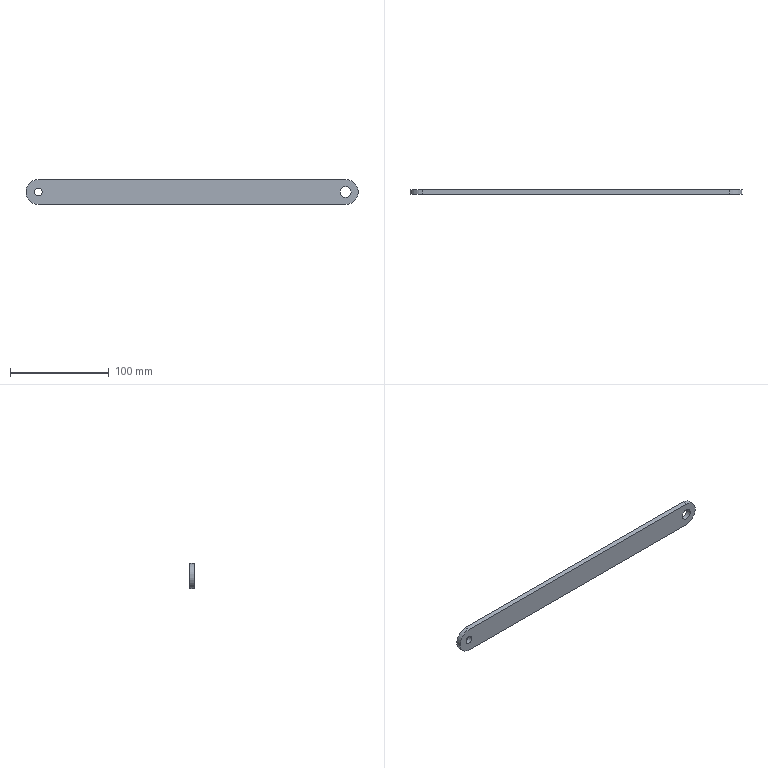Part | NX | features BREP 1 | 1 solid | 10 faces | box 336.55 x 4.763 x 25.4 mm | volume 39340 mm3 | cylinder 6 | plane 4 | commonest cylinder face diameters 8.128 x2 11.151 x2 25.4 x2
STEP:
#1=CARTESIAN_POINT('',(-155.575,0.,12.7));
#2=VERTEX_POINT('',#1);
#3=CARTESIAN_POINT('',(155.575,0.,12.7));
#4=VERTEX_POINT('',#3);
#5=CARTESIAN_POINT('',(-155.575,0.,12.7));
#6=DIRECTION('',(1.,0.,0.));
#7=VECTOR('',#6,1000.);
#8=LINE('',#5,#7);
#9=EDGE_CURVE('',#2,#4,#8,.T.);
#10=ORIENTED_EDGE('',*,*,#9,.T.);
#11=CARTESIAN_POINT('',(155.575,0.,-12.7));
#12=VERTEX_POINT('',#11);
#13=CARTESIAN_POINT('',(155.575,0.,0.));
#14=DIRECTION('',(0.,1.,0.));
#15=DIRECTION('',(0.,0.,1.));
#16=AXIS2_PLACEMENT_3D('',#13,#14,#15);
#17=CIRCLE('',#16,12.7);
#18=EDGE_CURVE('',#4,#12,#17,.T.);
#19=ORIENTED_EDGE('',*,*,#18,.T.);
#20=CARTESIAN_POINT('',(-155.575,0.,-12.7));
#21=VERTEX_POINT('',#20);
#22=CARTESIAN_POINT('',(155.575,0.,-12.7));
#23=DIRECTION('',(-1.,0.,0.));
#24=VECTOR('',#23,1000.);
#25=LINE('',#22,#24);
#26=EDGE_CURVE('',#12,#21,#25,.T.);
#27=ORIENTED_EDGE('',*,*,#26,.T.);
#28=CARTESIAN_POINT('',(-155.575,0.,0.));
#29=DIRECTION('',(0.,1.,0.));
#30=DIRECTION('',(0.,0.,-1.));
#31=AXIS2_PLACEMENT_3D('',#28,#29,#30);
#32=CIRCLE('',#31,12.7);
#33=EDGE_CURVE('',#21,#2,#32,.T.);
#34=ORIENTED_EDGE('',*,*,#33,.T.);
#35=EDGE_LOOP('',(#10,#19,#27,#34));
#36=FACE_BOUND('',#35,.T.);
#37=CARTESIAN_POINT('',(150.,0.,0.));
#38=VERTEX_POINT('',#37);
#39=CARTESIAN_POINT('',(161.15,0.,0.));
#40=VERTEX_POINT('',#39);
#41=CARTESIAN_POINT('',(155.575,0.,0.));
#42=DIRECTION('',(0.,-1.,0.));
#43=DIRECTION('',(-1.,0.,0.));
#44=AXIS2_PLACEMENT_3D('',#41,#42,#43);
#45=CIRCLE('',#44,5.575);
#46=EDGE_CURVE('',#38,#40,#45,.T.);
#47=ORIENTED_EDGE('',*,*,#46,.T.);
#48=CARTESIAN_POINT('',(155.575,0.,0.));
#49=DIRECTION('',(0.,-1.,0.));
#50=DIRECTION('',(1.,0.,0.));
#51=AXIS2_PLACEMENT_3D('',#48,#49,#50);
#52=CIRCLE('',#51,5.575);
#53=EDGE_CURVE('',#40,#38,#52,.T.);
#54=ORIENTED_EDGE('',*,*,#53,.T.);
#55=EDGE_LOOP('',(#47,#54));
#56=FACE_BOUND('',#55,.T.);
#57=CARTESIAN_POINT('',(-159.639,0.,0.));
#58=VERTEX_POINT('',#57);
#59=CARTESIAN_POINT('',(-151.511,0.,0.));
#60=VERTEX_POINT('',#59);
#61=CARTESIAN_POINT('',(-155.575,0.,0.));
#62=DIRECTION('',(0.,-1.,0.));
#63=DIRECTION('',(-1.,0.,0.));
#64=AXIS2_PLACEMENT_3D('',#61,#62,#63);
#65=CIRCLE('',#64,4.064);
#66=EDGE_CURVE('',#58,#60,#65,.T.);
#67=ORIENTED_EDGE('',*,*,#66,.T.);
#68=CARTESIAN_POINT('',(-155.575,0.,0.));
#69=DIRECTION('',(0.,-1.,0.));
#70=DIRECTION('',(1.,0.,0.));
#71=AXIS2_PLACEMENT_3D('',#68,#69,#70);
#72=CIRCLE('',#71,4.064);
#73=EDGE_CURVE('',#60,#58,#72,.T.);
#74=ORIENTED_EDGE('',*,*,#73,.T.);
#75=EDGE_LOOP('',(#67,#74));
#76=FACE_BOUND('',#75,.T.);
#77=CARTESIAN_POINT('',(0.,0.,0.));
#78=DIRECTION('',(0.,1.,0.));
#79=DIRECTION('',(1.,0.,0.));
#80=AXIS2_PLACEMENT_3D('',#77,#78,#79);
#81=PLANE('',#80);
#82=ADVANCED_FACE('',(#36,#56,#76),#81,.T.);
#83=CARTESIAN_POINT('',(-155.575,-4.763,-12.7));
#84=VERTEX_POINT('',#83);
#85=CARTESIAN_POINT('',(-155.575,0.,-12.7));
#86=DIRECTION('',(0.,-1.,0.));
#87=VECTOR('',#86,1000.);
#88=LINE('',#85,#87);
#89=EDGE_CURVE('',#21,#84,#88,.T.);
#90=ORIENTED_EDGE('',*,*,#89,.T.);
#91=CARTESIAN_POINT('',(-155.575,-4.763,12.7));
#92=VERTEX_POINT('',#91);
#93=CARTESIAN_POINT('',(-155.575,-4.763,0.));
#94=DIRECTION('',(0.,1.,0.));
#95=DIRECTION('',(0.,0.,-1.));
#96=AXIS2_PLACEMENT_3D('',#93,#94,#95);
#97=CIRCLE('',#96,12.7);
#98=EDGE_CURVE('',#84,#92,#97,.T.);
#99=ORIENTED_EDGE('',*,*,#98,.T.);
#100=CARTESIAN_POINT('',(-155.575,0.,12.7));
#101=DIRECTION('',(0.,-1.,0.));
#102=VECTOR('',#101,1000.);
#103=LINE('',#100,#102);
#104=EDGE_CURVE('',#2,#92,#103,.T.);
#105=ORIENTED_EDGE('',*,*,#104,.F.);
#106=ORIENTED_EDGE('',*,*,#33,.F.);
#107=EDGE_LOOP('',(#90,#99,#105,#106));
#108=FACE_BOUND('',#107,.T.);
#109=CARTESIAN_POINT('',(-155.575,-2.381,0.));
#110=DIRECTION('',(0.,1.,0.));
#111=DIRECTION('',(0.,0.,-1.));
#112=AXIS2_PLACEMENT_3D('',#109,#110,#111);
#113=CYLINDRICAL_SURFACE('',#112,12.7);
#114=ADVANCED_FACE('',(#108),#113,.T.);
#115=ORIENTED_EDGE('',*,*,#104,.T.);
#116=CARTESIAN_POINT('',(155.575,-4.763,12.7));
#117=VERTEX_POINT('',#116);
#118=CARTESIAN_POINT('',(-155.575,-4.763,12.7));
#119=DIRECTION('',(1.,0.,0.));
#120=VECTOR('',#119,1000.);
#121=LINE('',#118,#120);
#122=EDGE_CURVE('',#92,#117,#121,.T.);
#123=ORIENTED_EDGE('',*,*,#122,.T.);
#124=CARTESIAN_POINT('',(155.575,0.,12.7));
#125=DIRECTION('',(0.,-1.,0.));
#126=VECTOR('',#125,1000.);
#127=LINE('',#124,#126);
#128=EDGE_CURVE('',#4,#117,#127,.T.);
#129=ORIENTED_EDGE('',*,*,#128,.F.);
#130=ORIENTED_EDGE('',*,*,#9,.F.);
#131=EDGE_LOOP('',(#115,#123,#129,#130));
#132=FACE_BOUND('',#131,.T.);
#133=CARTESIAN_POINT('',(0.,-2.381,12.7));
#134=DIRECTION('',(0.,0.,1.));
#135=DIRECTION('',(1.,0.,0.));
#136=AXIS2_PLACEMENT_3D('',#133,#134,#135);
#137=PLANE('',#136);
#138=ADVANCED_FACE('',(#132),#137,.T.);
#139=ORIENTED_EDGE('',*,*,#128,.T.);
#140=CARTESIAN_POINT('',(155.575,-4.763,-12.7));
#141=VERTEX_POINT('',#140);
#142=CARTESIAN_POINT('',(155.575,-4.763,0.));
#143=DIRECTION('',(0.,1.,0.));
#144=DIRECTION('',(0.,0.,1.));
#145=AXIS2_PLACEMENT_3D('',#142,#143,#144);
#146=CIRCLE('',#145,12.7);
#147=EDGE_CURVE('',#117,#141,#146,.T.);
#148=ORIENTED_EDGE('',*,*,#147,.T.);
#149=CARTESIAN_POINT('',(155.575,0.,-12.7));
#150=DIRECTION('',(0.,-1.,0.));
#151=VECTOR('',#150,1000.);
#152=LINE('',#149,#151);
#153=EDGE_CURVE('',#12,#141,#152,.T.);
#154=ORIENTED_EDGE('',*,*,#153,.F.);
#155=ORIENTED_EDGE('',*,*,#18,.F.);
#156=EDGE_LOOP('',(#139,#148,#154,#155));
#157=FACE_BOUND('',#156,.T.);
#158=CARTESIAN_POINT('',(155.575,-2.381,0.));
#159=DIRECTION('',(0.,1.,0.));
#160=DIRECTION('',(0.,0.,1.));
#161=AXIS2_PLACEMENT_3D('',#158,#159,#160);
#162=CYLINDRICAL_SURFACE('',#161,12.7);
#163=ADVANCED_FACE('',(#157),#162,.T.);
#164=ORIENTED_EDGE('',*,*,#153,.T.);
#165=CARTESIAN_POINT('',(155.575,-4.763,-12.7));
#166=DIRECTION('',(-1.,0.,0.));
#167=VECTOR('',#166,1000.);
#168=LINE('',#165,#167);
#169=EDGE_CURVE('',#141,#84,#168,.T.);
#170=ORIENTED_EDGE('',*,*,#169,.T.);
#171=ORIENTED_EDGE('',*,*,#89,.F.);
#172=ORIENTED_EDGE('',*,*,#26,.F.);
#173=EDGE_LOOP('',(#164,#170,#171,#172));
#174=FACE_BOUND('',#173,.T.);
#175=CARTESIAN_POINT('',(0.,-2.381,-12.7));
#176=DIRECTION('',(0.,0.,-1.));
#177=DIRECTION('',(0.,-1.,0.));
#178=AXIS2_PLACEMENT_3D('',#175,#176,#177);
#179=PLANE('',#178);
#180=ADVANCED_FACE('',(#174),#179,.T.);
#181=ORIENTED_EDGE('',*,*,#169,.F.);
#182=ORIENTED_EDGE('',*,*,#147,.F.);
#183=ORIENTED_EDGE('',*,*,#122,.F.);
#184=ORIENTED_EDGE('',*,*,#98,.F.);
#185=EDGE_LOOP('',(#181,#182,#183,#184));
#186=FACE_BOUND('',#185,.T.);
#187=CARTESIAN_POINT('',(150.,-4.763,0.));
#188=VERTEX_POINT('',#187);
#189=CARTESIAN_POINT('',(161.15,-4.763,0.));
#190=VERTEX_POINT('',#189);
#191=CARTESIAN_POINT('',(155.575,-4.763,0.));
#192=DIRECTION('',(0.,-1.,0.));
#193=DIRECTION('',(-1.,0.,0.));
#194=AXIS2_PLACEMENT_3D('',#191,#192,#193);
#195=CIRCLE('',#194,5.575);
#196=EDGE_CURVE('',#188,#190,#195,.T.);
#197=ORIENTED_EDGE('',*,*,#196,.F.);
#198=CARTESIAN_POINT('',(155.575,-4.763,0.));
#199=DIRECTION('',(0.,-1.,0.));
#200=DIRECTION('',(1.,0.,0.));
#201=AXIS2_PLACEMENT_3D('',#198,#199,#200);
#202=CIRCLE('',#201,5.575);
#203=EDGE_CURVE('',#190,#188,#202,.T.);
#204=ORIENTED_EDGE('',*,*,#203,.F.);
#205=EDGE_LOOP('',(#197,#204));
#206=FACE_BOUND('',#205,.T.);
#207=CARTESIAN_POINT('',(-159.639,-4.763,0.));
#208=VERTEX_POINT('',#207);
#209=CARTESIAN_POINT('',(-151.511,-4.763,0.));
#210=VERTEX_POINT('',#209);
#211=CARTESIAN_POINT('',(-155.575,-4.763,0.));
#212=DIRECTION('',(0.,-1.,0.));
#213=DIRECTION('',(-1.,0.,0.));
#214=AXIS2_PLACEMENT_3D('',#211,#212,#213);
#215=CIRCLE('',#214,4.064);
#216=EDGE_CURVE('',#208,#210,#215,.T.);
#217=ORIENTED_EDGE('',*,*,#216,.F.);
#218=CARTESIAN_POINT('',(-155.575,-4.763,0.));
#219=DIRECTION('',(0.,-1.,0.));
#220=DIRECTION('',(1.,0.,0.));
#221=AXIS2_PLACEMENT_3D('',#218,#219,#220);
#222=CIRCLE('',#221,4.064);
#223=EDGE_CURVE('',#210,#208,#222,.T.);
#224=ORIENTED_EDGE('',*,*,#223,.F.);
#225=EDGE_LOOP('',(#217,#224));
#226=FACE_BOUND('',#225,.T.);
#227=CARTESIAN_POINT('',(0.,-4.763,0.));
#228=DIRECTION('',(0.,1.,0.));
#229=DIRECTION('',(1.,0.,0.));
#230=AXIS2_PLACEMENT_3D('',#227,#228,#229);
#231=PLANE('',#230);
#232=ADVANCED_FACE('',(#186,#206,#226),#231,.F.);
#233=CARTESIAN_POINT('',(161.15,0.,0.));
#234=DIRECTION('',(0.,-1.,0.));
#235=VECTOR('',#234,1000.);
#236=LINE('',#233,#235);
#237=EDGE_CURVE('',#190,#40,#236,.F.);
#238=ORIENTED_EDGE('',*,*,#237,.F.);
#239=ORIENTED_EDGE('',*,*,#203,.T.);
#240=CARTESIAN_POINT('',(150.,0.,0.));
#241=DIRECTION('',(0.,-1.,0.));
#242=VECTOR('',#241,1000.);
#243=LINE('',#240,#242);
#244=EDGE_CURVE('',#188,#38,#243,.F.);
#245=ORIENTED_EDGE('',*,*,#244,.T.);
#246=ORIENTED_EDGE('',*,*,#53,.F.);
#247=EDGE_LOOP('',(#238,#239,#245,#246));
#248=FACE_BOUND('',#247,.T.);
#249=CARTESIAN_POINT('',(155.575,0.,0.));
#250=DIRECTION('',(0.,-1.,0.));
#251=DIRECTION('',(1.,0.,0.));
#252=AXIS2_PLACEMENT_3D('',#249,#250,#251);
#253=CYLINDRICAL_SURFACE('',#252,5.575);
#254=ADVANCED_FACE('',(#248),#253,.F.);
#255=ORIENTED_EDGE('',*,*,#244,.F.);
#256=ORIENTED_EDGE('',*,*,#196,.T.);
#257=ORIENTED_EDGE('',*,*,#237,.T.);
#258=ORIENTED_EDGE('',*,*,#46,.F.);
#259=EDGE_LOOP('',(#255,#256,#257,#258));
#260=FACE_BOUND('',#259,.T.);
#261=CARTESIAN_POINT('',(155.575,0.,0.));
#262=DIRECTION('',(0.,-1.,0.));
#263=DIRECTION('',(1.,0.,0.));
#264=AXIS2_PLACEMENT_3D('',#261,#262,#263);
#265=CYLINDRICAL_SURFACE('',#264,5.575);
#266=ADVANCED_FACE('',(#260),#265,.F.);
#267=CARTESIAN_POINT('',(-151.511,0.,0.));
#268=DIRECTION('',(0.,-1.,0.));
#269=VECTOR('',#268,1000.);
#270=LINE('',#267,#269);
#271=EDGE_CURVE('',#210,#60,#270,.F.);
#272=ORIENTED_EDGE('',*,*,#271,.F.);
#273=ORIENTED_EDGE('',*,*,#223,.T.);
#274=CARTESIAN_POINT('',(-159.639,0.,0.));
#275=DIRECTION('',(0.,-1.,0.));
#276=VECTOR('',#275,1000.);
#277=LINE('',#274,#276);
#278=EDGE_CURVE('',#208,#58,#277,.F.);
#279=ORIENTED_EDGE('',*,*,#278,.T.);
#280=ORIENTED_EDGE('',*,*,#73,.F.);
#281=EDGE_LOOP('',(#272,#273,#279,#280));
#282=FACE_BOUND('',#281,.T.);
#283=CARTESIAN_POINT('',(-155.575,0.,0.));
#284=DIRECTION('',(0.,-1.,0.));
#285=DIRECTION('',(1.,0.,0.));
#286=AXIS2_PLACEMENT_3D('',#283,#284,#285);
#287=CYLINDRICAL_SURFACE('',#286,4.064);
#288=ADVANCED_FACE('',(#282),#287,.F.);
#289=ORIENTED_EDGE('',*,*,#278,.F.);
#290=ORIENTED_EDGE('',*,*,#216,.T.);
#291=ORIENTED_EDGE('',*,*,#271,.T.);
#292=ORIENTED_EDGE('',*,*,#66,.F.);
#293=EDGE_LOOP('',(#289,#290,#291,#292));
#294=FACE_BOUND('',#293,.T.);
#295=CARTESIAN_POINT('',(-155.575,0.,0.));
#296=DIRECTION('',(0.,-1.,0.));
#297=DIRECTION('',(1.,0.,0.));
#298=AXIS2_PLACEMENT_3D('',#295,#296,#297);
#299=CYLINDRICAL_SURFACE('',#298,4.064);
#300=ADVANCED_FACE('',(#294),#299,.F.);
#301=CLOSED_SHELL('',(#82,#114,#138,#163,#180,#232,#254,#266,#288,#300));
#302=MANIFOLD_SOLID_BREP('',#301);
#303=(LENGTH_UNIT()NAMED_UNIT(*)SI_UNIT(.MILLI.,.METRE.));
#304=UNCERTAINTY_MEASURE_WITH_UNIT(LENGTH_MEASURE(0.00001),#303,'','');
#305=(NAMED_UNIT(*)PLANE_ANGLE_UNIT()SI_UNIT($,.RADIAN.));
#306=(NAMED_UNIT(*)SI_UNIT($,.STERADIAN.)SOLID_ANGLE_UNIT());
#307=(GEOMETRIC_REPRESENTATION_CONTEXT(3)GLOBAL_UNCERTAINTY_ASSIGNED_CONTEXT((#304))GLOBAL_UNIT_ASSIGNED_CONTEXT((#303,#305,#306))REPRESENTATION_CONTEXT('',''));
#308=ADVANCED_BREP_SHAPE_REPRESENTATION('',(#302),#307);